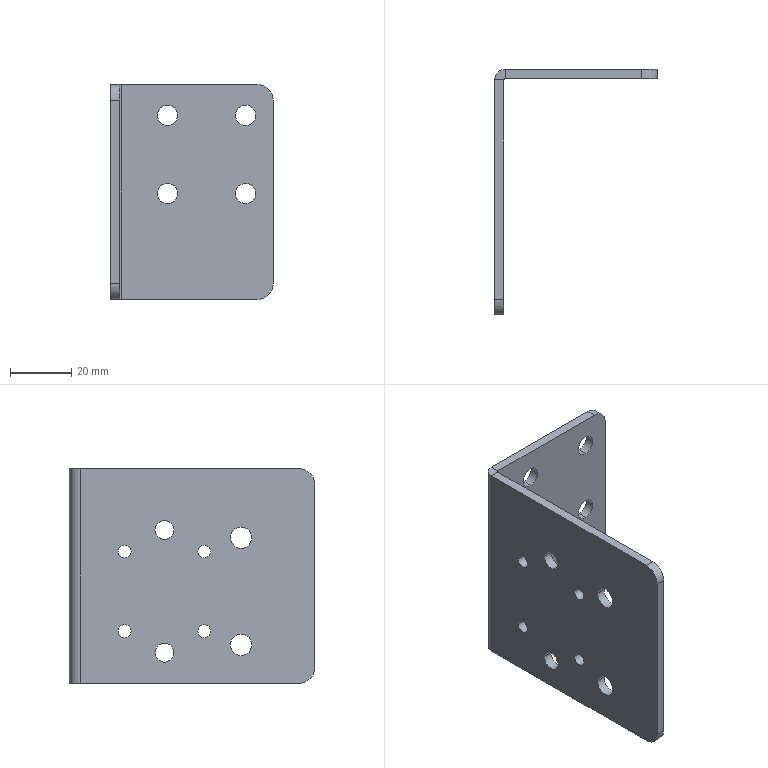Part | SolidWorks | features ICE 11, Fillet 2, ExtruThin 1, FlatPattern 1, FlattenBends 1, ProcessBends 1, SheetMetal 1 | 1 solid | 42 faces | box 53 x 80 x 70 mm | volume 26067 mm3 | cylinder 30 | plane 12 | commonest cylinder face diameters 4.2 x8 6.6 x8 7 x5 6.2 x4 10 x4 1 x1
STEP:
#1=CARTESIAN_POINT('',(0.,122.1,20.));
#2=VERTEX_POINT('',#1);
#3=CARTESIAN_POINT('',(0.,115.9,20.));
#4=VERTEX_POINT('',#3);
#5=CARTESIAN_POINT('',(0.,119.,20.));
#6=DIRECTION('',(-1.,0.,0.));
#7=DIRECTION('',(0.,-1.,0.));
#8=AXIS2_PLACEMENT_3D('',#5,#6,#7);
#9=CIRCLE('',#8,3.1);
#10=EDGE_CURVE('',#2,#4,#9,.T.);
#11=ORIENTED_EDGE('',*,*,#10,.T.);
#12=CARTESIAN_POINT('',(3.,115.9,20.));
#13=VERTEX_POINT('',#12);
#14=CARTESIAN_POINT('',(-7.,115.9,20.));
#15=DIRECTION('',(1.,0.,0.));
#16=VECTOR('',#15,1000.);
#17=LINE('',#14,#16);
#18=EDGE_CURVE('',#4,#13,#17,.T.);
#19=ORIENTED_EDGE('',*,*,#18,.T.);
#20=CARTESIAN_POINT('',(3.,122.1,20.));
#21=VERTEX_POINT('',#20);
#22=CARTESIAN_POINT('',(3.,119.,20.));
#23=DIRECTION('',(1.,0.,0.));
#24=DIRECTION('',(0.,1.,0.));
#25=AXIS2_PLACEMENT_3D('',#22,#23,#24);
#26=CIRCLE('',#25,3.1);
#27=EDGE_CURVE('',#13,#21,#26,.T.);
#28=ORIENTED_EDGE('',*,*,#27,.T.);
#29=CARTESIAN_POINT('',(-7.,122.1,20.));
#30=DIRECTION('',(1.,0.,0.));
#31=VECTOR('',#30,1000.);
#32=LINE('',#29,#31);
#33=EDGE_CURVE('',#2,#21,#32,.T.);
#34=ORIENTED_EDGE('',*,*,#33,.F.);
#35=EDGE_LOOP('',(#11,#19,#28,#34));
#36=FACE_OUTER_BOUND('',#35,.T.);
#37=CARTESIAN_POINT('',(-7.,119.,20.));
#38=DIRECTION('',(1.,0.,0.));
#39=DIRECTION('',(0.,1.,0.));
#40=AXIS2_PLACEMENT_3D('',#37,#38,#39);
#41=CYLINDRICAL_SURFACE('',#40,3.1);
#42=ADVANCED_FACE('',(#36),#41,.F.);
#43=CARTESIAN_POINT('',(0.,97.5,17.5));
#44=VERTEX_POINT('',#43);
#45=CARTESIAN_POINT('',(0.,90.5,17.5));
#46=VERTEX_POINT('',#45);
#47=CARTESIAN_POINT('',(0.,94.,17.5));
#48=DIRECTION('',(-1.,0.,0.));
#49=DIRECTION('',(0.,-1.,0.));
#50=AXIS2_PLACEMENT_3D('',#47,#48,#49);
#51=CIRCLE('',#50,3.5);
#52=EDGE_CURVE('',#44,#46,#51,.T.);
#53=ORIENTED_EDGE('',*,*,#52,.T.);
#54=CARTESIAN_POINT('',(3.,90.5,17.5));
#55=VERTEX_POINT('',#54);
#56=CARTESIAN_POINT('',(-7.,90.5,17.5));
#57=DIRECTION('',(1.,0.,0.));
#58=VECTOR('',#57,1000.);
#59=LINE('',#56,#58);
#60=EDGE_CURVE('',#46,#55,#59,.T.);
#61=ORIENTED_EDGE('',*,*,#60,.T.);
#62=CARTESIAN_POINT('',(3.,97.5,17.5));
#63=VERTEX_POINT('',#62);
#64=CARTESIAN_POINT('',(3.,94.,17.5));
#65=DIRECTION('',(1.,0.,0.));
#66=DIRECTION('',(0.,1.,0.));
#67=AXIS2_PLACEMENT_3D('',#64,#65,#66);
#68=CIRCLE('',#67,3.5);
#69=EDGE_CURVE('',#55,#63,#68,.T.);
#70=ORIENTED_EDGE('',*,*,#69,.T.);
#71=CARTESIAN_POINT('',(-7.,97.5,17.5));
#72=DIRECTION('',(1.,0.,0.));
#73=VECTOR('',#72,1000.);
#74=LINE('',#71,#73);
#75=EDGE_CURVE('',#44,#63,#74,.T.);
#76=ORIENTED_EDGE('',*,*,#75,.F.);
#77=EDGE_LOOP('',(#53,#61,#70,#76));
#78=FACE_OUTER_BOUND('',#77,.T.);
#79=CARTESIAN_POINT('',(-7.,94.,17.5));
#80=DIRECTION('',(1.,0.,0.));
#81=DIRECTION('',(0.,1.,0.));
#82=AXIS2_PLACEMENT_3D('',#79,#80,#81);
#83=CYLINDRICAL_SURFACE('',#82,3.5);
#84=ADVANCED_FACE('',(#78),#83,.F.);
#85=CARTESIAN_POINT('',(0.,97.5,-17.5));
#86=VERTEX_POINT('',#85);
#87=CARTESIAN_POINT('',(0.,90.5,-17.5));
#88=VERTEX_POINT('',#87);
#89=CARTESIAN_POINT('',(0.,94.,-17.5));
#90=DIRECTION('',(-1.,0.,0.));
#91=DIRECTION('',(0.,-1.,0.));
#92=AXIS2_PLACEMENT_3D('',#89,#90,#91);
#93=CIRCLE('',#92,3.5);
#94=EDGE_CURVE('',#86,#88,#93,.T.);
#95=ORIENTED_EDGE('',*,*,#94,.T.);
#96=CARTESIAN_POINT('',(3.,90.5,-17.5));
#97=VERTEX_POINT('',#96);
#98=CARTESIAN_POINT('',(-7.,90.5,-17.5));
#99=DIRECTION('',(1.,0.,0.));
#100=VECTOR('',#99,1000.);
#101=LINE('',#98,#100);
#102=EDGE_CURVE('',#88,#97,#101,.T.);
#103=ORIENTED_EDGE('',*,*,#102,.T.);
#104=CARTESIAN_POINT('',(3.,97.5,-17.5));
#105=VERTEX_POINT('',#104);
#106=CARTESIAN_POINT('',(3.,94.,-17.5));
#107=DIRECTION('',(1.,0.,0.));
#108=DIRECTION('',(0.,1.,0.));
#109=AXIS2_PLACEMENT_3D('',#106,#107,#108);
#110=CIRCLE('',#109,3.5);
#111=EDGE_CURVE('',#97,#105,#110,.T.);
#112=ORIENTED_EDGE('',*,*,#111,.T.);
#113=CARTESIAN_POINT('',(-7.,97.5,-17.5));
#114=DIRECTION('',(1.,0.,0.));
#115=VECTOR('',#114,1000.);
#116=LINE('',#113,#115);
#117=EDGE_CURVE('',#86,#105,#116,.T.);
#118=ORIENTED_EDGE('',*,*,#117,.F.);
#119=EDGE_LOOP('',(#95,#103,#112,#118));
#120=FACE_OUTER_BOUND('',#119,.T.);
#121=CARTESIAN_POINT('',(-7.,94.,-17.5));
#122=DIRECTION('',(1.,0.,0.));
#123=DIRECTION('',(0.,1.,0.));
#124=AXIS2_PLACEMENT_3D('',#121,#122,#123);
#125=CYLINDRICAL_SURFACE('',#124,3.5);
#126=ADVANCED_FACE('',(#120),#125,.F.);
#127=CARTESIAN_POINT('',(0.,122.1,-20.));
#128=VERTEX_POINT('',#127);
#129=CARTESIAN_POINT('',(0.,115.9,-20.));
#130=VERTEX_POINT('',#129);
#131=CARTESIAN_POINT('',(0.,119.,-20.));
#132=DIRECTION('',(-1.,0.,0.));
#133=DIRECTION('',(0.,-1.,0.));
#134=AXIS2_PLACEMENT_3D('',#131,#132,#133);
#135=CIRCLE('',#134,3.1);
#136=EDGE_CURVE('',#128,#130,#135,.T.);
#137=ORIENTED_EDGE('',*,*,#136,.T.);
#138=CARTESIAN_POINT('',(3.,115.9,-20.));
#139=VERTEX_POINT('',#138);
#140=CARTESIAN_POINT('',(-7.,115.9,-20.));
#141=DIRECTION('',(1.,0.,0.));
#142=VECTOR('',#141,1000.);
#143=LINE('',#140,#142);
#144=EDGE_CURVE('',#130,#139,#143,.T.);
#145=ORIENTED_EDGE('',*,*,#144,.T.);
#146=CARTESIAN_POINT('',(3.,122.1,-20.));
#147=VERTEX_POINT('',#146);
#148=CARTESIAN_POINT('',(3.,119.,-20.));
#149=DIRECTION('',(1.,0.,0.));
#150=DIRECTION('',(0.,1.,0.));
#151=AXIS2_PLACEMENT_3D('',#148,#149,#150);
#152=CIRCLE('',#151,3.1);
#153=EDGE_CURVE('',#139,#147,#152,.T.);
#154=ORIENTED_EDGE('',*,*,#153,.T.);
#155=CARTESIAN_POINT('',(-7.,122.1,-20.));
#156=DIRECTION('',(1.,0.,0.));
#157=VECTOR('',#156,1000.);
#158=LINE('',#155,#157);
#159=EDGE_CURVE('',#128,#147,#158,.T.);
#160=ORIENTED_EDGE('',*,*,#159,.F.);
#161=EDGE_LOOP('',(#137,#145,#154,#160));
#162=FACE_OUTER_BOUND('',#161,.T.);
#163=CARTESIAN_POINT('',(-7.,119.,-20.));
#164=DIRECTION('',(1.,0.,0.));
#165=DIRECTION('',(0.,1.,0.));
#166=AXIS2_PLACEMENT_3D('',#163,#164,#165);
#167=CYLINDRICAL_SURFACE('',#166,3.1);
#168=ADVANCED_FACE('',(#162),#167,.F.);
#169=CARTESIAN_POINT('',(0.,108.1,13.));
#170=VERTEX_POINT('',#169);
#171=CARTESIAN_POINT('',(0.,103.9,13.));
#172=VERTEX_POINT('',#171);
#173=CARTESIAN_POINT('',(0.,106.,13.));
#174=DIRECTION('',(-1.,0.,0.));
#175=DIRECTION('',(0.,-1.,0.));
#176=AXIS2_PLACEMENT_3D('',#173,#174,#175);
#177=CIRCLE('',#176,2.1);
#178=EDGE_CURVE('',#170,#172,#177,.T.);
#179=ORIENTED_EDGE('',*,*,#178,.T.);
#180=CARTESIAN_POINT('',(3.,103.9,13.));
#181=VERTEX_POINT('',#180);
#182=CARTESIAN_POINT('',(-7.,103.9,13.));
#183=DIRECTION('',(1.,0.,0.));
#184=VECTOR('',#183,1000.);
#185=LINE('',#182,#184);
#186=EDGE_CURVE('',#172,#181,#185,.T.);
#187=ORIENTED_EDGE('',*,*,#186,.T.);
#188=CARTESIAN_POINT('',(3.,108.1,13.));
#189=VERTEX_POINT('',#188);
#190=CARTESIAN_POINT('',(3.,106.,13.));
#191=DIRECTION('',(1.,0.,0.));
#192=DIRECTION('',(0.,1.,0.));
#193=AXIS2_PLACEMENT_3D('',#190,#191,#192);
#194=CIRCLE('',#193,2.1);
#195=EDGE_CURVE('',#181,#189,#194,.T.);
#196=ORIENTED_EDGE('',*,*,#195,.T.);
#197=CARTESIAN_POINT('',(-7.,108.1,13.));
#198=DIRECTION('',(1.,0.,0.));
#199=VECTOR('',#198,1000.);
#200=LINE('',#197,#199);
#201=EDGE_CURVE('',#170,#189,#200,.T.);
#202=ORIENTED_EDGE('',*,*,#201,.F.);
#203=EDGE_LOOP('',(#179,#187,#196,#202));
#204=FACE_OUTER_BOUND('',#203,.T.);
#205=CARTESIAN_POINT('',(-7.,106.,13.));
#206=DIRECTION('',(1.,0.,0.));
#207=DIRECTION('',(0.,1.,0.));
#208=AXIS2_PLACEMENT_3D('',#205,#206,#207);
#209=CYLINDRICAL_SURFACE('',#208,2.1);
#210=ADVANCED_FACE('',(#204),#209,.F.);
#211=CARTESIAN_POINT('',(0.,108.1,-13.));
#212=VERTEX_POINT('',#211);
#213=CARTESIAN_POINT('',(0.,103.9,-13.));
#214=VERTEX_POINT('',#213);
#215=CARTESIAN_POINT('',(0.,106.,-13.));
#216=DIRECTION('',(-1.,0.,0.));
#217=DIRECTION('',(0.,-1.,0.));
#218=AXIS2_PLACEMENT_3D('',#215,#216,#217);
#219=CIRCLE('',#218,2.1);
#220=EDGE_CURVE('',#212,#214,#219,.T.);
#221=ORIENTED_EDGE('',*,*,#220,.T.);
#222=CARTESIAN_POINT('',(3.,103.9,-13.));
#223=VERTEX_POINT('',#222);
#224=CARTESIAN_POINT('',(-7.,103.9,-13.));
#225=DIRECTION('',(1.,0.,0.));
#226=VECTOR('',#225,1000.);
#227=LINE('',#224,#226);
#228=EDGE_CURVE('',#214,#223,#227,.T.);
#229=ORIENTED_EDGE('',*,*,#228,.T.);
#230=CARTESIAN_POINT('',(3.,108.1,-13.));
#231=VERTEX_POINT('',#230);
#232=CARTESIAN_POINT('',(3.,106.,-13.));
#233=DIRECTION('',(1.,0.,0.));
#234=DIRECTION('',(0.,1.,0.));
#235=AXIS2_PLACEMENT_3D('',#232,#233,#234);
#236=CIRCLE('',#235,2.1);
#237=EDGE_CURVE('',#223,#231,#236,.T.);
#238=ORIENTED_EDGE('',*,*,#237,.T.);
#239=CARTESIAN_POINT('',(-7.,108.1,-13.));
#240=DIRECTION('',(1.,0.,0.));
#241=VECTOR('',#240,1000.);
#242=LINE('',#239,#241);
#243=EDGE_CURVE('',#212,#231,#242,.T.);
#244=ORIENTED_EDGE('',*,*,#243,.F.);
#245=EDGE_LOOP('',(#221,#229,#238,#244));
#246=FACE_OUTER_BOUND('',#245,.T.);
#247=CARTESIAN_POINT('',(-7.,106.,-13.));
#248=DIRECTION('',(1.,0.,0.));
#249=DIRECTION('',(0.,1.,0.));
#250=AXIS2_PLACEMENT_3D('',#247,#248,#249);
#251=CYLINDRICAL_SURFACE('',#250,2.1);
#252=ADVANCED_FACE('',(#246),#251,.F.);
#253=CARTESIAN_POINT('',(0.,134.1,-13.));
#254=VERTEX_POINT('',#253);
#255=CARTESIAN_POINT('',(0.,129.9,-13.));
#256=VERTEX_POINT('',#255);
#257=CARTESIAN_POINT('',(0.,132.,-13.));
#258=DIRECTION('',(-1.,0.,0.));
#259=DIRECTION('',(0.,-1.,0.));
#260=AXIS2_PLACEMENT_3D('',#257,#258,#259);
#261=CIRCLE('',#260,2.1);
#262=EDGE_CURVE('',#254,#256,#261,.T.);
#263=ORIENTED_EDGE('',*,*,#262,.T.);
#264=CARTESIAN_POINT('',(3.,129.9,-13.));
#265=VERTEX_POINT('',#264);
#266=CARTESIAN_POINT('',(-7.,129.9,-13.));
#267=DIRECTION('',(1.,0.,0.));
#268=VECTOR('',#267,1000.);
#269=LINE('',#266,#268);
#270=EDGE_CURVE('',#256,#265,#269,.T.);
#271=ORIENTED_EDGE('',*,*,#270,.T.);
#272=CARTESIAN_POINT('',(3.,134.1,-13.));
#273=VERTEX_POINT('',#272);
#274=CARTESIAN_POINT('',(3.,132.,-13.));
#275=DIRECTION('',(1.,0.,0.));
#276=DIRECTION('',(0.,1.,0.));
#277=AXIS2_PLACEMENT_3D('',#274,#275,#276);
#278=CIRCLE('',#277,2.1);
#279=EDGE_CURVE('',#265,#273,#278,.T.);
#280=ORIENTED_EDGE('',*,*,#279,.T.);
#281=CARTESIAN_POINT('',(-7.,134.1,-13.));
#282=DIRECTION('',(1.,0.,0.));
#283=VECTOR('',#282,1000.);
#284=LINE('',#281,#283);
#285=EDGE_CURVE('',#254,#273,#284,.T.);
#286=ORIENTED_EDGE('',*,*,#285,.F.);
#287=EDGE_LOOP('',(#263,#271,#280,#286));
#288=FACE_OUTER_BOUND('',#287,.T.);
#289=CARTESIAN_POINT('',(-7.,132.,-13.));
#290=DIRECTION('',(1.,0.,0.));
#291=DIRECTION('',(0.,1.,0.));
#292=AXIS2_PLACEMENT_3D('',#289,#290,#291);
#293=CYLINDRICAL_SURFACE('',#292,2.1);
#294=ADVANCED_FACE('',(#288),#293,.F.);
#295=CARTESIAN_POINT('',(0.,134.1,13.));
#296=VERTEX_POINT('',#295);
#297=CARTESIAN_POINT('',(0.,129.9,13.));
#298=VERTEX_POINT('',#297);
#299=CARTESIAN_POINT('',(0.,132.,13.));
#300=DIRECTION('',(-1.,0.,0.));
#301=DIRECTION('',(0.,-1.,0.));
#302=AXIS2_PLACEMENT_3D('',#299,#300,#301);
#303=CIRCLE('',#302,2.1);
#304=EDGE_CURVE('',#296,#298,#303,.T.);
#305=ORIENTED_EDGE('',*,*,#304,.T.);
#306=CARTESIAN_POINT('',(3.,129.9,13.));
#307=VERTEX_POINT('',#306);
#308=CARTESIAN_POINT('',(-7.,129.9,13.));
#309=DIRECTION('',(1.,0.,0.));
#310=VECTOR('',#309,1000.);
#311=LINE('',#308,#310);
#312=EDGE_CURVE('',#298,#307,#311,.T.);
#313=ORIENTED_EDGE('',*,*,#312,.T.);
#314=CARTESIAN_POINT('',(3.,134.1,13.));
#315=VERTEX_POINT('',#314);
#316=CARTESIAN_POINT('',(3.,132.,13.));
#317=DIRECTION('',(1.,0.,0.));
#318=DIRECTION('',(0.,1.,0.));
#319=AXIS2_PLACEMENT_3D('',#316,#317,#318);
#320=CIRCLE('',#319,2.1);
#321=EDGE_CURVE('',#307,#315,#320,.T.);
#322=ORIENTED_EDGE('',*,*,#321,.T.);
#323=CARTESIAN_POINT('',(-7.,134.1,13.));
#324=DIRECTION('',(1.,0.,0.));
#325=VECTOR('',#324,1000.);
#326=LINE('',#323,#325);
#327=EDGE_CURVE('',#296,#315,#326,.T.);
#328=ORIENTED_EDGE('',*,*,#327,.F.);
#329=EDGE_LOOP('',(#305,#313,#322,#328));
#330=FACE_OUTER_BOUND('',#329,.T.);
#331=CARTESIAN_POINT('',(-7.,132.,13.));
#332=DIRECTION('',(1.,0.,0.));
#333=DIRECTION('',(0.,1.,0.));
#334=AXIS2_PLACEMENT_3D('',#331,#332,#333);
#335=CYLINDRICAL_SURFACE('',#334,2.1);
#336=ADVANCED_FACE('',(#330),#335,.F.);
#337=CARTESIAN_POINT('',(44.,147.,26.7));
#338=VERTEX_POINT('',#337);
#339=CARTESIAN_POINT('',(44.,147.,33.3));
#340=VERTEX_POINT('',#339);
#341=CARTESIAN_POINT('',(44.,147.,30.));
#342=DIRECTION('',(0.,1.,0.));
#343=DIRECTION('',(-1.,0.,0.));
#344=AXIS2_PLACEMENT_3D('',#341,#342,#343);
#345=CIRCLE('',#344,3.3);
#346=EDGE_CURVE('',#338,#340,#345,.T.);
#347=ORIENTED_EDGE('',*,*,#346,.F.);
#348=CARTESIAN_POINT('',(44.,150.,26.7));
#349=VERTEX_POINT('',#348);
#350=CARTESIAN_POINT('',(44.,140.,26.7));
#351=DIRECTION('',(0.,1.,0.));
#352=VECTOR('',#351,1000.);
#353=LINE('',#350,#352);
#354=EDGE_CURVE('',#338,#349,#353,.T.);
#355=ORIENTED_EDGE('',*,*,#354,.T.);
#356=CARTESIAN_POINT('',(44.,150.,33.3));
#357=VERTEX_POINT('',#356);
#358=CARTESIAN_POINT('',(44.,150.,30.));
#359=DIRECTION('',(0.,1.,0.));
#360=DIRECTION('',(0.,0.,1.));
#361=AXIS2_PLACEMENT_3D('',#358,#359,#360);
#362=CIRCLE('',#361,3.3);
#363=EDGE_CURVE('',#349,#357,#362,.T.);
#364=ORIENTED_EDGE('',*,*,#363,.T.);
#365=CARTESIAN_POINT('',(44.,140.,33.3));
#366=DIRECTION('',(0.,1.,0.));
#367=VECTOR('',#366,1000.);
#368=LINE('',#365,#367);
#369=EDGE_CURVE('',#340,#357,#368,.T.);
#370=ORIENTED_EDGE('',*,*,#369,.F.);
#371=EDGE_LOOP('',(#347,#355,#364,#370));
#372=FACE_OUTER_BOUND('',#371,.T.);
#373=CARTESIAN_POINT('',(44.,140.,30.));
#374=DIRECTION('',(0.,1.,0.));
#375=DIRECTION('',(0.,0.,1.));
#376=AXIS2_PLACEMENT_3D('',#373,#374,#375);
#377=CYLINDRICAL_SURFACE('',#376,3.3);
#378=ADVANCED_FACE('',(#372),#377,.F.);
#379=CARTESIAN_POINT('',(44.,147.,1.2));
#380=VERTEX_POINT('',#379);
#381=CARTESIAN_POINT('',(44.,147.,7.8));
#382=VERTEX_POINT('',#381);
#383=CARTESIAN_POINT('',(44.,147.,4.5));
#384=DIRECTION('',(0.,1.,0.));
#385=DIRECTION('',(-1.,0.,0.));
#386=AXIS2_PLACEMENT_3D('',#383,#384,#385);
#387=CIRCLE('',#386,3.3);
#388=EDGE_CURVE('',#380,#382,#387,.T.);
#389=ORIENTED_EDGE('',*,*,#388,.F.);
#390=CARTESIAN_POINT('',(44.,150.,1.2));
#391=VERTEX_POINT('',#390);
#392=CARTESIAN_POINT('',(44.,140.,1.2));
#393=DIRECTION('',(0.,1.,0.));
#394=VECTOR('',#393,1000.);
#395=LINE('',#392,#394);
#396=EDGE_CURVE('',#380,#391,#395,.T.);
#397=ORIENTED_EDGE('',*,*,#396,.T.);
#398=CARTESIAN_POINT('',(44.,150.,7.8));
#399=VERTEX_POINT('',#398);
#400=CARTESIAN_POINT('',(44.,150.,4.5));
#401=DIRECTION('',(0.,1.,0.));
#402=DIRECTION('',(0.,0.,1.));
#403=AXIS2_PLACEMENT_3D('',#400,#401,#402);
#404=CIRCLE('',#403,3.3);
#405=EDGE_CURVE('',#391,#399,#404,.T.);
#406=ORIENTED_EDGE('',*,*,#405,.T.);
#407=CARTESIAN_POINT('',(44.,140.,7.8));
#408=DIRECTION('',(0.,1.,0.));
#409=VECTOR('',#408,1000.);
#410=LINE('',#407,#409);
#411=EDGE_CURVE('',#382,#399,#410,.T.);
#412=ORIENTED_EDGE('',*,*,#411,.F.);
#413=EDGE_LOOP('',(#389,#397,#406,#412));
#414=FACE_OUTER_BOUND('',#413,.T.);
#415=CARTESIAN_POINT('',(44.,140.,4.5));
#416=DIRECTION('',(0.,1.,0.));
#417=DIRECTION('',(0.,0.,1.));
#418=AXIS2_PLACEMENT_3D('',#415,#416,#417);
#419=CYLINDRICAL_SURFACE('',#418,3.3);
#420=ADVANCED_FACE('',(#414),#419,.F.);
#421=CARTESIAN_POINT('',(18.5,147.,1.2));
#422=VERTEX_POINT('',#421);
#423=CARTESIAN_POINT('',(18.5,147.,7.8));
#424=VERTEX_POINT('',#423);
#425=CARTESIAN_POINT('',(18.5,147.,4.5));
#426=DIRECTION('',(0.,1.,0.));
#427=DIRECTION('',(-1.,0.,0.));
#428=AXIS2_PLACEMENT_3D('',#425,#426,#427);
#429=CIRCLE('',#428,3.3);
#430=EDGE_CURVE('',#422,#424,#429,.T.);
#431=ORIENTED_EDGE('',*,*,#430,.F.);
#432=CARTESIAN_POINT('',(18.5,150.,1.2));
#433=VERTEX_POINT('',#432);
#434=CARTESIAN_POINT('',(18.5,140.,1.2));
#435=DIRECTION('',(0.,1.,0.));
#436=VECTOR('',#435,1000.);
#437=LINE('',#434,#436);
#438=EDGE_CURVE('',#422,#433,#437,.T.);
#439=ORIENTED_EDGE('',*,*,#438,.T.);
#440=CARTESIAN_POINT('',(18.5,150.,7.8));
#441=VERTEX_POINT('',#440);
#442=CARTESIAN_POINT('',(18.5,150.,4.5));
#443=DIRECTION('',(0.,1.,0.));
#444=DIRECTION('',(0.,0.,1.));
#445=AXIS2_PLACEMENT_3D('',#442,#443,#444);
#446=CIRCLE('',#445,3.3);
#447=EDGE_CURVE('',#433,#441,#446,.T.);
#448=ORIENTED_EDGE('',*,*,#447,.T.);
#449=CARTESIAN_POINT('',(18.5,140.,7.8));
#450=DIRECTION('',(0.,1.,0.));
#451=VECTOR('',#450,1000.);
#452=LINE('',#449,#451);
#453=EDGE_CURVE('',#424,#441,#452,.T.);
#454=ORIENTED_EDGE('',*,*,#453,.F.);
#455=EDGE_LOOP('',(#431,#439,#448,#454));
#456=FACE_OUTER_BOUND('',#455,.T.);
#457=CARTESIAN_POINT('',(18.5,140.,4.5));
#458=DIRECTION('',(0.,1.,0.));
#459=DIRECTION('',(0.,0.,1.));
#460=AXIS2_PLACEMENT_3D('',#457,#458,#459);
#461=CYLINDRICAL_SURFACE('',#460,3.3);
#462=ADVANCED_FACE('',(#456),#461,.F.);
#463=CARTESIAN_POINT('',(18.5,147.,26.7));
#464=VERTEX_POINT('',#463);
#465=CARTESIAN_POINT('',(18.5,147.,33.3));
#466=VERTEX_POINT('',#465);
#467=CARTESIAN_POINT('',(18.5,147.,30.));
#468=DIRECTION('',(0.,1.,0.));
#469=DIRECTION('',(-1.,0.,0.));
#470=AXIS2_PLACEMENT_3D('',#467,#468,#469);
#471=CIRCLE('',#470,3.3);
#472=EDGE_CURVE('',#464,#466,#471,.T.);
#473=ORIENTED_EDGE('',*,*,#472,.F.);
#474=CARTESIAN_POINT('',(18.5,150.,26.7));
#475=VERTEX_POINT('',#474);
#476=CARTESIAN_POINT('',(18.5,140.,26.7));
#477=DIRECTION('',(0.,1.,0.));
#478=VECTOR('',#477,1000.);
#479=LINE('',#476,#478);
#480=EDGE_CURVE('',#464,#475,#479,.T.);
#481=ORIENTED_EDGE('',*,*,#480,.T.);
#482=CARTESIAN_POINT('',(18.5,150.,33.3));
#483=VERTEX_POINT('',#482);
#484=CARTESIAN_POINT('',(18.5,150.,30.));
#485=DIRECTION('',(0.,1.,0.));
#486=DIRECTION('',(0.,0.,1.));
#487=AXIS2_PLACEMENT_3D('',#484,#485,#486);
#488=CIRCLE('',#487,3.3);
#489=EDGE_CURVE('',#475,#483,#488,.T.);
#490=ORIENTED_EDGE('',*,*,#489,.T.);
#491=CARTESIAN_POINT('',(18.5,140.,33.3));
#492=DIRECTION('',(0.,1.,0.));
#493=VECTOR('',#492,1000.);
#494=LINE('',#491,#493);
#495=EDGE_CURVE('',#466,#483,#494,.T.);
#496=ORIENTED_EDGE('',*,*,#495,.F.);
#497=EDGE_LOOP('',(#473,#481,#490,#496));
#498=FACE_OUTER_BOUND('',#497,.T.);
#499=CARTESIAN_POINT('',(18.5,140.,30.));
#500=DIRECTION('',(0.,1.,0.));
#501=DIRECTION('',(0.,0.,1.));
#502=AXIS2_PLACEMENT_3D('',#499,#500,#501);
#503=CYLINDRICAL_SURFACE('',#502,3.3);
#504=ADVANCED_FACE('',(#498),#503,.F.);
#505=ORIENTED_EDGE('',*,*,#480,.F.);
#506=CARTESIAN_POINT('',(18.5,147.,30.));
#507=DIRECTION('',(0.,1.,0.));
#508=DIRECTION('',(-1.,0.,0.));
#509=AXIS2_PLACEMENT_3D('',#506,#507,#508);
#510=CIRCLE('',#509,3.3);
#511=EDGE_CURVE('',#466,#464,#510,.T.);
#512=ORIENTED_EDGE('',*,*,#511,.F.);
#513=ORIENTED_EDGE('',*,*,#495,.T.);
#514=CARTESIAN_POINT('',(18.5,150.,30.));
#515=DIRECTION('',(0.,1.,0.));
#516=DIRECTION('',(0.,0.,1.));
#517=AXIS2_PLACEMENT_3D('',#514,#515,#516);
#518=CIRCLE('',#517,3.3);
#519=EDGE_CURVE('',#483,#475,#518,.T.);
#520=ORIENTED_EDGE('',*,*,#519,.T.);
#521=EDGE_LOOP('',(#505,#512,#513,#520));
#522=FACE_OUTER_BOUND('',#521,.T.);
#523=CARTESIAN_POINT('',(18.5,140.,30.));
#524=DIRECTION('',(0.,1.,0.));
#525=DIRECTION('',(0.,0.,1.));
#526=AXIS2_PLACEMENT_3D('',#523,#524,#525);
#527=CYLINDRICAL_SURFACE('',#526,3.3);
#528=ADVANCED_FACE('',(#522),#527,.F.);
#529=ORIENTED_EDGE('',*,*,#438,.F.);
#530=CARTESIAN_POINT('',(18.5,147.,4.5));
#531=DIRECTION('',(0.,1.,0.));
#532=DIRECTION('',(-1.,0.,0.));
#533=AXIS2_PLACEMENT_3D('',#530,#531,#532);
#534=CIRCLE('',#533,3.3);
#535=EDGE_CURVE('',#424,#422,#534,.T.);
#536=ORIENTED_EDGE('',*,*,#535,.F.);
#537=ORIENTED_EDGE('',*,*,#453,.T.);
#538=CARTESIAN_POINT('',(18.5,150.,4.5));
#539=DIRECTION('',(0.,1.,0.));
#540=DIRECTION('',(0.,0.,1.));
#541=AXIS2_PLACEMENT_3D('',#538,#539,#540);
#542=CIRCLE('',#541,3.3);
#543=EDGE_CURVE('',#441,#433,#542,.T.);
#544=ORIENTED_EDGE('',*,*,#543,.T.);
#545=EDGE_LOOP('',(#529,#536,#537,#544));
#546=FACE_OUTER_BOUND('',#545,.T.);
#547=CARTESIAN_POINT('',(18.5,140.,4.5));
#548=DIRECTION('',(0.,1.,0.));
#549=DIRECTION('',(0.,0.,1.));
#550=AXIS2_PLACEMENT_3D('',#547,#548,#549);
#551=CYLINDRICAL_SURFACE('',#550,3.3);
#552=ADVANCED_FACE('',(#546),#551,.F.);
#553=ORIENTED_EDGE('',*,*,#396,.F.);
#554=CARTESIAN_POINT('',(44.,147.,4.5));
#555=DIRECTION('',(0.,1.,0.));
#556=DIRECTION('',(-1.,0.,0.));
#557=AXIS2_PLACEMENT_3D('',#554,#555,#556);
#558=CIRCLE('',#557,3.3);
#559=EDGE_CURVE('',#382,#380,#558,.T.);
#560=ORIENTED_EDGE('',*,*,#559,.F.);
#561=ORIENTED_EDGE('',*,*,#411,.T.);
#562=CARTESIAN_POINT('',(44.,150.,4.5));
#563=DIRECTION('',(0.,1.,0.));
#564=DIRECTION('',(0.,0.,1.));
#565=AXIS2_PLACEMENT_3D('',#562,#563,#564);
#566=CIRCLE('',#565,3.3);
#567=EDGE_CURVE('',#399,#391,#566,.T.);
#568=ORIENTED_EDGE('',*,*,#567,.T.);
#569=EDGE_LOOP('',(#553,#560,#561,#568));
#570=FACE_OUTER_BOUND('',#569,.T.);
#571=CARTESIAN_POINT('',(44.,140.,4.5));
#572=DIRECTION('',(0.,1.,0.));
#573=DIRECTION('',(0.,0.,1.));
#574=AXIS2_PLACEMENT_3D('',#571,#572,#573);
#575=CYLINDRICAL_SURFACE('',#574,3.3);
#576=ADVANCED_FACE('',(#570),#575,.F.);
#577=ORIENTED_EDGE('',*,*,#354,.F.);
#578=CARTESIAN_POINT('',(44.,147.,30.));
#579=DIRECTION('',(0.,1.,0.));
#580=DIRECTION('',(-1.,0.,0.));
#581=AXIS2_PLACEMENT_3D('',#578,#579,#580);
#582=CIRCLE('',#581,3.3);
#583=EDGE_CURVE('',#340,#338,#582,.T.);
#584=ORIENTED_EDGE('',*,*,#583,.F.);
#585=ORIENTED_EDGE('',*,*,#369,.T.);
#586=CARTESIAN_POINT('',(44.,150.,30.));
#587=DIRECTION('',(0.,1.,0.));
#588=DIRECTION('',(0.,0.,1.));
#589=AXIS2_PLACEMENT_3D('',#586,#587,#588);
#590=CIRCLE('',#589,3.3);
#591=EDGE_CURVE('',#357,#349,#590,.T.);
#592=ORIENTED_EDGE('',*,*,#591,.T.);
#593=EDGE_LOOP('',(#577,#584,#585,#592));
#594=FACE_OUTER_BOUND('',#593,.T.);
#595=CARTESIAN_POINT('',(44.,140.,30.));
#596=DIRECTION('',(0.,1.,0.));
#597=DIRECTION('',(0.,0.,1.));
#598=AXIS2_PLACEMENT_3D('',#595,#596,#597);
#599=CYLINDRICAL_SURFACE('',#598,3.3);
#600=ADVANCED_FACE('',(#594),#599,.F.);
#601=CARTESIAN_POINT('',(53.,147.,-25.));
#602=VERTEX_POINT('',#601);
#603=CARTESIAN_POINT('',(53.,150.,-25.));
#604=VERTEX_POINT('',#603);
#605=CARTESIAN_POINT('',(53.,-21.467,-25.));
#606=DIRECTION('',(0.,1.,0.));
#607=VECTOR('',#606,1000.);
#608=LINE('',#605,#607);
#609=EDGE_CURVE('',#602,#604,#608,.T.);
#610=ORIENTED_EDGE('',*,*,#609,.T.);
#611=CARTESIAN_POINT('',(53.,150.,35.));
#612=VERTEX_POINT('',#611);
#613=CARTESIAN_POINT('',(53.,150.,30.));
#614=DIRECTION('',(0.,0.,1.));
#615=VECTOR('',#614,1000.);
#616=LINE('',#613,#615);
#617=EDGE_CURVE('',#604,#612,#616,.T.);
#618=ORIENTED_EDGE('',*,*,#617,.T.);
#619=CARTESIAN_POINT('',(53.,147.,35.));
#620=VERTEX_POINT('',#619);
#621=CARTESIAN_POINT('',(53.,-21.467,35.));
#622=DIRECTION('',(0.,1.,0.));
#623=VECTOR('',#622,1000.);
#624=LINE('',#621,#623);
#625=EDGE_CURVE('',#620,#612,#624,.T.);
#626=ORIENTED_EDGE('',*,*,#625,.F.);
#627=CARTESIAN_POINT('',(53.,147.,30.));
#628=DIRECTION('',(0.,0.,-1.));
#629=VECTOR('',#628,1000.);
#630=LINE('',#627,#629);
#631=EDGE_CURVE('',#620,#602,#630,.T.);
#632=ORIENTED_EDGE('',*,*,#631,.T.);
#633=EDGE_LOOP('',(#610,#618,#626,#632));
#634=FACE_OUTER_BOUND('',#633,.T.);
#635=CARTESIAN_POINT('',(53.,-21.467,30.));
#636=DIRECTION('',(1.,0.,0.));
#637=DIRECTION('',(0.,1.,0.));
#638=AXIS2_PLACEMENT_3D('',#635,#636,#637);
#639=PLANE('',#638);
#640=ADVANCED_FACE('',(#634),#639,.T.);
#641=CARTESIAN_POINT('',(48.,150.,40.));
#642=VERTEX_POINT('',#641);
#643=CARTESIAN_POINT('',(48.,150.,35.));
#644=DIRECTION('',(0.,1.,0.));
#645=DIRECTION('',(0.,0.,1.));
#646=AXIS2_PLACEMENT_3D('',#643,#644,#645);
#647=CIRCLE('',#646,5.);
#648=EDGE_CURVE('',#642,#612,#647,.T.);
#649=ORIENTED_EDGE('',*,*,#648,.F.);
#650=CARTESIAN_POINT('',(48.,147.,40.));
#651=VERTEX_POINT('',#650);
#652=CARTESIAN_POINT('',(48.,-21.467,40.));
#653=DIRECTION('',(0.,1.,0.));
#654=VECTOR('',#653,1000.);
#655=LINE('',#652,#654);
#656=EDGE_CURVE('',#651,#642,#655,.T.);
#657=ORIENTED_EDGE('',*,*,#656,.F.);
#658=CARTESIAN_POINT('',(48.,147.,35.));
#659=DIRECTION('',(0.,-1.,0.));
#660=DIRECTION('',(-1.,0.,0.));
#661=AXIS2_PLACEMENT_3D('',#658,#659,#660);
#662=CIRCLE('',#661,5.);
#663=EDGE_CURVE('',#620,#651,#662,.T.);
#664=ORIENTED_EDGE('',*,*,#663,.F.);
#665=ORIENTED_EDGE('',*,*,#625,.T.);
#666=EDGE_LOOP('',(#649,#657,#664,#665));
#667=FACE_OUTER_BOUND('',#666,.T.);
#668=CARTESIAN_POINT('',(48.,-21.467,35.));
#669=DIRECTION('',(0.,1.,0.));
#670=DIRECTION('',(-1.,0.,0.));
#671=AXIS2_PLACEMENT_3D('',#668,#669,#670);
#672=CYLINDRICAL_SURFACE('',#671,5.);
#673=ADVANCED_FACE('',(#667),#672,.T.);
#674=CARTESIAN_POINT('',(48.,150.,-30.));
#675=VERTEX_POINT('',#674);
#676=CARTESIAN_POINT('',(48.,150.,-25.));
#677=DIRECTION('',(0.,1.,0.));
#678=DIRECTION('',(0.,0.,1.));
#679=AXIS2_PLACEMENT_3D('',#676,#677,#678);
#680=CIRCLE('',#679,5.);
#681=EDGE_CURVE('',#604,#675,#680,.T.);
#682=ORIENTED_EDGE('',*,*,#681,.F.);
#683=ORIENTED_EDGE('',*,*,#609,.F.);
#684=CARTESIAN_POINT('',(48.,147.,-30.));
#685=VERTEX_POINT('',#684);
#686=CARTESIAN_POINT('',(48.,147.,-25.));
#687=DIRECTION('',(0.,-1.,0.));
#688=DIRECTION('',(-1.,0.,0.));
#689=AXIS2_PLACEMENT_3D('',#686,#687,#688);
#690=CIRCLE('',#689,5.);
#691=EDGE_CURVE('',#685,#602,#690,.T.);
#692=ORIENTED_EDGE('',*,*,#691,.F.);
#693=CARTESIAN_POINT('',(48.,-21.467,-30.));
#694=DIRECTION('',(0.,1.,0.));
#695=VECTOR('',#694,1000.);
#696=LINE('',#693,#695);
#697=EDGE_CURVE('',#685,#675,#696,.T.);
#698=ORIENTED_EDGE('',*,*,#697,.T.);
#699=EDGE_LOOP('',(#682,#683,#692,#698));
#700=FACE_OUTER_BOUND('',#699,.T.);
#701=CARTESIAN_POINT('',(48.,-21.467,-25.));
#702=DIRECTION('',(0.,1.,0.));
#703=DIRECTION('',(-1.,0.,0.));
#704=AXIS2_PLACEMENT_3D('',#701,#702,#703);
#705=CYLINDRICAL_SURFACE('',#704,5.);
#706=ADVANCED_FACE('',(#700),#705,.T.);
#707=CARTESIAN_POINT('',(3.5,147.,-30.));
#708=VERTEX_POINT('',#707);
#709=CARTESIAN_POINT('',(3.5,150.,-30.));
#710=VERTEX_POINT('',#709);
#711=CARTESIAN_POINT('',(3.5,-21.467,-30.));
#712=DIRECTION('',(0.,1.,0.));
#713=VECTOR('',#712,1000.);
#714=LINE('',#711,#713);
#715=EDGE_CURVE('',#708,#710,#714,.T.);
#716=ORIENTED_EDGE('',*,*,#715,.T.);
#717=CARTESIAN_POINT('',(3.,150.,-30.));
#718=DIRECTION('',(-1.,0.,0.));
#719=VECTOR('',#718,1000.);
#720=LINE('',#717,#719);
#721=EDGE_CURVE('',#675,#710,#720,.T.);
#722=ORIENTED_EDGE('',*,*,#721,.F.);
#723=ORIENTED_EDGE('',*,*,#697,.F.);
#724=CARTESIAN_POINT('',(53.,147.,-30.));
#725=DIRECTION('',(-1.,0.,0.));
#726=VECTOR('',#725,1000.);
#727=LINE('',#724,#726);
#728=EDGE_CURVE('',#685,#708,#727,.T.);
#729=ORIENTED_EDGE('',*,*,#728,.T.);
#730=EDGE_LOOP('',(#716,#722,#723,#729));
#731=FACE_OUTER_BOUND('',#730,.T.);
#732=CARTESIAN_POINT('',(53.,-21.467,-30.));
#733=DIRECTION('',(0.,0.,-1.));
#734=DIRECTION('',(0.,1.,0.));
#735=AXIS2_PLACEMENT_3D('',#732,#733,#734);
#736=PLANE('',#735);
#737=ADVANCED_FACE('',(#731),#736,.T.);
#738=CARTESIAN_POINT('',(3.5,150.,40.));
#739=VERTEX_POINT('',#738);
#740=CARTESIAN_POINT('',(3.5,150.,-30.));
#741=DIRECTION('',(0.,0.,-1.));
#742=VECTOR('',#741,1000.);
#743=LINE('',#740,#742);
#744=EDGE_CURVE('',#739,#710,#743,.T.);
#745=ORIENTED_EDGE('',*,*,#744,.F.);
#746=CARTESIAN_POINT('',(53.,150.,40.));
#747=DIRECTION('',(-1.,0.,0.));
#748=VECTOR('',#747,1000.);
#749=LINE('',#746,#748);
#750=EDGE_CURVE('',#642,#739,#749,.T.);
#751=ORIENTED_EDGE('',*,*,#750,.F.);
#752=ORIENTED_EDGE('',*,*,#648,.T.);
#753=ORIENTED_EDGE('',*,*,#617,.F.);
#754=ORIENTED_EDGE('',*,*,#681,.T.);
#755=ORIENTED_EDGE('',*,*,#721,.T.);
#756=EDGE_LOOP('',(#745,#751,#752,#753,#754,#755));
#757=FACE_OUTER_BOUND('',#756,.T.);
#758=ORIENTED_EDGE('',*,*,#591,.F.);
#759=ORIENTED_EDGE('',*,*,#363,.F.);
#760=EDGE_LOOP('',(#758,#759));
#761=FACE_BOUND('',#760,.T.);
#762=ORIENTED_EDGE('',*,*,#567,.F.);
#763=ORIENTED_EDGE('',*,*,#405,.F.);
#764=EDGE_LOOP('',(#762,#763));
#765=FACE_BOUND('',#764,.T.);
#766=ORIENTED_EDGE('',*,*,#543,.F.);
#767=ORIENTED_EDGE('',*,*,#447,.F.);
#768=EDGE_LOOP('',(#766,#767));
#769=FACE_BOUND('',#768,.T.);
#770=ORIENTED_EDGE('',*,*,#519,.F.);
#771=ORIENTED_EDGE('',*,*,#489,.F.);
#772=EDGE_LOOP('',(#770,#771));
#773=FACE_BOUND('',#772,.T.);
#774=CARTESIAN_POINT('',(0.,150.,0.));
#775=DIRECTION('',(0.,1.,0.));
#776=DIRECTION('',(0.,0.,1.));
#777=AXIS2_PLACEMENT_3D('',#774,#775,#776);
#778=PLANE('',#777);
#779=ADVANCED_FACE('',(#757,#761,#765,#769,#773),#778,.T.);
#780=ORIENTED_EDGE('',*,*,#656,.T.);
#781=ORIENTED_EDGE('',*,*,#750,.T.);
#782=CARTESIAN_POINT('',(3.5,147.,40.));
#783=VERTEX_POINT('',#782);
#784=CARTESIAN_POINT('',(3.5,-21.467,40.));
#785=DIRECTION('',(0.,1.,0.));
#786=VECTOR('',#785,1000.);
#787=LINE('',#784,#786);
#788=EDGE_CURVE('',#783,#739,#787,.T.);
#789=ORIENTED_EDGE('',*,*,#788,.F.);
#790=CARTESIAN_POINT('',(3.,147.,40.));
#791=DIRECTION('',(-1.,0.,0.));
#792=VECTOR('',#791,1000.);
#793=LINE('',#790,#792);
#794=EDGE_CURVE('',#651,#783,#793,.T.);
#795=ORIENTED_EDGE('',*,*,#794,.F.);
#796=EDGE_LOOP('',(#780,#781,#789,#795));
#797=FACE_OUTER_BOUND('',#796,.T.);
#798=CARTESIAN_POINT('',(3.,-21.467,40.));
#799=DIRECTION('',(0.,0.,1.));
#800=DIRECTION('',(0.,-1.,0.));
#801=AXIS2_PLACEMENT_3D('',#798,#799,#800);
#802=PLANE('',#801);
#803=ADVANCED_FACE('',(#797),#802,.T.);
#804=ORIENTED_EDGE('',*,*,#583,.T.);
#805=ORIENTED_EDGE('',*,*,#346,.T.);
#806=EDGE_LOOP('',(#804,#805));
#807=FACE_BOUND('',#806,.T.);
#808=ORIENTED_EDGE('',*,*,#559,.T.);
#809=ORIENTED_EDGE('',*,*,#388,.T.);
#810=EDGE_LOOP('',(#808,#809));
#811=FACE_BOUND('',#810,.T.);
#812=ORIENTED_EDGE('',*,*,#535,.T.);
#813=ORIENTED_EDGE('',*,*,#430,.T.);
#814=EDGE_LOOP('',(#812,#813));
#815=FACE_BOUND('',#814,.T.);
#816=ORIENTED_EDGE('',*,*,#511,.T.);
#817=ORIENTED_EDGE('',*,*,#472,.T.);
#818=EDGE_LOOP('',(#816,#817));
#819=FACE_BOUND('',#818,.T.);
#820=ORIENTED_EDGE('',*,*,#794,.T.);
#821=CARTESIAN_POINT('',(3.5,147.,-30.));
#822=DIRECTION('',(0.,0.,-1.));
#823=VECTOR('',#822,1000.);
#824=LINE('',#821,#823);
#825=EDGE_CURVE('',#783,#708,#824,.T.);
#826=ORIENTED_EDGE('',*,*,#825,.T.);
#827=ORIENTED_EDGE('',*,*,#728,.F.);
#828=ORIENTED_EDGE('',*,*,#691,.T.);
#829=ORIENTED_EDGE('',*,*,#631,.F.);
#830=ORIENTED_EDGE('',*,*,#663,.T.);
#831=EDGE_LOOP('',(#820,#826,#827,#828,#829,#830));
#832=FACE_OUTER_BOUND('',#831,.T.);
#833=CARTESIAN_POINT('',(53.,147.,30.));
#834=DIRECTION('',(0.,1.,0.));
#835=DIRECTION('',(-1.,0.,0.));
#836=AXIS2_PLACEMENT_3D('',#833,#834,#835);
#837=PLANE('',#836);
#838=ADVANCED_FACE('',(#807,#811,#815,#819,#832),#837,.F.);
#839=ORIENTED_EDGE('',*,*,#52,.F.);
#840=CARTESIAN_POINT('',(0.,94.,17.5));
#841=DIRECTION('',(-1.,0.,0.));
#842=DIRECTION('',(0.,-1.,0.));
#843=AXIS2_PLACEMENT_3D('',#840,#841,#842);
#844=CIRCLE('',#843,3.5);
#845=EDGE_CURVE('',#46,#44,#844,.T.);
#846=ORIENTED_EDGE('',*,*,#845,.F.);
#847=EDGE_LOOP('',(#839,#846));
#848=FACE_BOUND('',#847,.T.);
#849=ORIENTED_EDGE('',*,*,#94,.F.);
#850=CARTESIAN_POINT('',(0.,94.,-17.5));
#851=DIRECTION('',(-1.,0.,0.));
#852=DIRECTION('',(0.,-1.,0.));
#853=AXIS2_PLACEMENT_3D('',#850,#851,#852);
#854=CIRCLE('',#853,3.5);
#855=EDGE_CURVE('',#88,#86,#854,.T.);
#856=ORIENTED_EDGE('',*,*,#855,.F.);
#857=EDGE_LOOP('',(#849,#856));
#858=FACE_BOUND('',#857,.T.);
#859=ORIENTED_EDGE('',*,*,#136,.F.);
#860=CARTESIAN_POINT('',(0.,119.,-20.));
#861=DIRECTION('',(-1.,0.,0.));
#862=DIRECTION('',(0.,-1.,0.));
#863=AXIS2_PLACEMENT_3D('',#860,#861,#862);
#864=CIRCLE('',#863,3.1);
#865=EDGE_CURVE('',#130,#128,#864,.T.);
#866=ORIENTED_EDGE('',*,*,#865,.F.);
#867=EDGE_LOOP('',(#859,#866));
#868=FACE_BOUND('',#867,.T.);
#869=ORIENTED_EDGE('',*,*,#178,.F.);
#870=CARTESIAN_POINT('',(0.,106.,13.));
#871=DIRECTION('',(-1.,0.,0.));
#872=DIRECTION('',(0.,-1.,0.));
#873=AXIS2_PLACEMENT_3D('',#870,#871,#872);
#874=CIRCLE('',#873,2.1);
#875=EDGE_CURVE('',#172,#170,#874,.T.);
#876=ORIENTED_EDGE('',*,*,#875,.F.);
#877=EDGE_LOOP('',(#869,#876));
#878=FACE_BOUND('',#877,.T.);
#879=ORIENTED_EDGE('',*,*,#220,.F.);
#880=CARTESIAN_POINT('',(0.,106.,-13.));
#881=DIRECTION('',(-1.,0.,0.));
#882=DIRECTION('',(0.,-1.,0.));
#883=AXIS2_PLACEMENT_3D('',#880,#881,#882);
#884=CIRCLE('',#883,2.1);
#885=EDGE_CURVE('',#214,#212,#884,.T.);
#886=ORIENTED_EDGE('',*,*,#885,.F.);
#887=EDGE_LOOP('',(#879,#886));
#888=FACE_BOUND('',#887,.T.);
#889=ORIENTED_EDGE('',*,*,#262,.F.);
#890=CARTESIAN_POINT('',(0.,132.,-13.));
#891=DIRECTION('',(-1.,0.,0.));
#892=DIRECTION('',(0.,-1.,0.));
#893=AXIS2_PLACEMENT_3D('',#890,#891,#892);
#894=CIRCLE('',#893,2.1);
#895=EDGE_CURVE('',#256,#254,#894,.T.);
#896=ORIENTED_EDGE('',*,*,#895,.F.);
#897=EDGE_LOOP('',(#889,#896));
#898=FACE_BOUND('',#897,.T.);
#899=ORIENTED_EDGE('',*,*,#304,.F.);
#900=CARTESIAN_POINT('',(0.,132.,13.));
#901=DIRECTION('',(-1.,0.,0.));
#902=DIRECTION('',(0.,-1.,0.));
#903=AXIS2_PLACEMENT_3D('',#900,#901,#902);
#904=CIRCLE('',#903,2.1);
#905=EDGE_CURVE('',#298,#296,#904,.T.);
#906=ORIENTED_EDGE('',*,*,#905,.F.);
#907=EDGE_LOOP('',(#899,#906));
#908=FACE_BOUND('',#907,.T.);
#909=ORIENTED_EDGE('',*,*,#10,.F.);
#910=CARTESIAN_POINT('',(0.,119.,20.));
#911=DIRECTION('',(-1.,0.,0.));
#912=DIRECTION('',(0.,-1.,0.));
#913=AXIS2_PLACEMENT_3D('',#910,#911,#912);
#914=CIRCLE('',#913,3.1);
#915=EDGE_CURVE('',#4,#2,#914,.T.);
#916=ORIENTED_EDGE('',*,*,#915,.F.);
#917=EDGE_LOOP('',(#909,#916));
#918=FACE_BOUND('',#917,.T.);
#919=CARTESIAN_POINT('',(0.,146.5,40.));
#920=VERTEX_POINT('',#919);
#921=CARTESIAN_POINT('',(0.,75.,40.));
#922=VERTEX_POINT('',#921);
#923=CARTESIAN_POINT('',(0.,150.,40.));
#924=DIRECTION('',(0.,-1.,0.));
#925=VECTOR('',#924,1000.);
#926=LINE('',#923,#925);
#927=EDGE_CURVE('',#920,#922,#926,.T.);
#928=ORIENTED_EDGE('',*,*,#927,.F.);
#929=CARTESIAN_POINT('',(0.,146.5,-30.));
#930=VERTEX_POINT('',#929);
#931=CARTESIAN_POINT('',(0.,146.5,-30.));
#932=DIRECTION('',(0.,0.,-1.));
#933=VECTOR('',#932,1000.);
#934=LINE('',#931,#933);
#935=EDGE_CURVE('',#920,#930,#934,.T.);
#936=ORIENTED_EDGE('',*,*,#935,.T.);
#937=CARTESIAN_POINT('',(0.,75.,-30.));
#938=VERTEX_POINT('',#937);
#939=CARTESIAN_POINT('',(0.,139.,-30.));
#940=DIRECTION('',(0.,1.,0.));
#941=VECTOR('',#940,1000.);
#942=LINE('',#939,#941);
#943=EDGE_CURVE('',#938,#930,#942,.T.);
#944=ORIENTED_EDGE('',*,*,#943,.F.);
#945=CARTESIAN_POINT('',(0.,70.,-25.));
#946=VERTEX_POINT('',#945);
#947=CARTESIAN_POINT('',(0.,75.,-25.));
#948=DIRECTION('',(-1.,0.,0.));
#949=DIRECTION('',(0.,-1.,0.));
#950=AXIS2_PLACEMENT_3D('',#947,#948,#949);
#951=CIRCLE('',#950,5.);
#952=EDGE_CURVE('',#938,#946,#951,.T.);
#953=ORIENTED_EDGE('',*,*,#952,.T.);
#954=CARTESIAN_POINT('',(0.,70.,35.));
#955=VERTEX_POINT('',#954);
#956=CARTESIAN_POINT('',(0.,70.,-60.));
#957=DIRECTION('',(0.,0.,-1.));
#958=VECTOR('',#957,1000.);
#959=LINE('',#956,#958);
#960=EDGE_CURVE('',#955,#946,#959,.T.);
#961=ORIENTED_EDGE('',*,*,#960,.F.);
#962=CARTESIAN_POINT('',(0.,75.,35.));
#963=DIRECTION('',(-1.,0.,0.));
#964=DIRECTION('',(0.,-1.,0.));
#965=AXIS2_PLACEMENT_3D('',#962,#963,#964);
#966=CIRCLE('',#965,5.);
#967=EDGE_CURVE('',#955,#922,#966,.T.);
#968=ORIENTED_EDGE('',*,*,#967,.T.);
#969=EDGE_LOOP('',(#928,#936,#944,#953,#961,#968));
#970=FACE_OUTER_BOUND('',#969,.T.);
#971=CARTESIAN_POINT('',(0.,139.,-60.));
#972=DIRECTION('',(-1.,0.,0.));
#973=DIRECTION('',(0.,-1.,0.));
#974=AXIS2_PLACEMENT_3D('',#971,#972,#973);
#975=PLANE('',#974);
#976=ADVANCED_FACE('',(#848,#858,#868,#878,#888,#898,#908,#918,#970),#975,.T.);
#977=CARTESIAN_POINT('',(3.,94.,17.5));
#978=DIRECTION('',(1.,0.,0.));
#979=DIRECTION('',(0.,1.,0.));
#980=AXIS2_PLACEMENT_3D('',#977,#978,#979);
#981=CIRCLE('',#980,3.5);
#982=EDGE_CURVE('',#63,#55,#981,.T.);
#983=ORIENTED_EDGE('',*,*,#982,.F.);
#984=ORIENTED_EDGE('',*,*,#69,.F.);
#985=EDGE_LOOP('',(#983,#984));
#986=FACE_BOUND('',#985,.T.);
#987=CARTESIAN_POINT('',(3.,94.,-17.5));
#988=DIRECTION('',(1.,0.,0.));
#989=DIRECTION('',(0.,1.,0.));
#990=AXIS2_PLACEMENT_3D('',#987,#988,#989);
#991=CIRCLE('',#990,3.5);
#992=EDGE_CURVE('',#105,#97,#991,.T.);
#993=ORIENTED_EDGE('',*,*,#992,.F.);
#994=ORIENTED_EDGE('',*,*,#111,.F.);
#995=EDGE_LOOP('',(#993,#994));
#996=FACE_BOUND('',#995,.T.);
#997=CARTESIAN_POINT('',(3.,119.,-20.));
#998=DIRECTION('',(1.,0.,0.));
#999=DIRECTION('',(0.,1.,0.));
#1000=AXIS2_PLACEMENT_3D('',#997,#998,#999);
#1001=CIRCLE('',#1000,3.1);
#1002=EDGE_CURVE('',#147,#139,#1001,.T.);
#1003=ORIENTED_EDGE('',*,*,#1002,.F.);
#1004=ORIENTED_EDGE('',*,*,#153,.F.);
#1005=EDGE_LOOP('',(#1003,#1004));
#1006=FACE_BOUND('',#1005,.T.);
#1007=CARTESIAN_POINT('',(3.,106.,13.));
#1008=DIRECTION('',(1.,0.,0.));
#1009=DIRECTION('',(0.,1.,0.));
#1010=AXIS2_PLACEMENT_3D('',#1007,#1008,#1009);
#1011=CIRCLE('',#1010,2.1);
#1012=EDGE_CURVE('',#189,#181,#1011,.T.);
#1013=ORIENTED_EDGE('',*,*,#1012,.F.);
#1014=ORIENTED_EDGE('',*,*,#195,.F.);
#1015=EDGE_LOOP('',(#1013,#1014));
#1016=FACE_BOUND('',#1015,.T.);
#1017=CARTESIAN_POINT('',(3.,106.,-13.));
#1018=DIRECTION('',(1.,0.,0.));
#1019=DIRECTION('',(0.,1.,0.));
#1020=AXIS2_PLACEMENT_3D('',#1017,#1018,#1019);
#1021=CIRCLE('',#1020,2.1);
#1022=EDGE_CURVE('',#231,#223,#1021,.T.);
#1023=ORIENTED_EDGE('',*,*,#1022,.F.);
#1024=ORIENTED_EDGE('',*,*,#237,.F.);
#1025=EDGE_LOOP('',(#1023,#1024));
#1026=FACE_BOUND('',#1025,.T.);
#1027=CARTESIAN_POINT('',(3.,132.,-13.));
#1028=DIRECTION('',(1.,0.,0.));
#1029=DIRECTION('',(0.,1.,0.));
#1030=AXIS2_PLACEMENT_3D('',#1027,#1028,#1029);
#1031=CIRCLE('',#1030,2.1);
#1032=EDGE_CURVE('',#273,#265,#1031,.T.);
#1033=ORIENTED_EDGE('',*,*,#1032,.F.);
#1034=ORIENTED_EDGE('',*,*,#279,.F.);
#1035=EDGE_LOOP('',(#1033,#1034));
#1036=FACE_BOUND('',#1035,.T.);
#1037=CARTESIAN_POINT('',(3.,132.,13.));
#1038=DIRECTION('',(1.,0.,0.));
#1039=DIRECTION('',(0.,1.,0.));
#1040=AXIS2_PLACEMENT_3D('',#1037,#1038,#1039);
#1041=CIRCLE('',#1040,2.1);
#1042=EDGE_CURVE('',#315,#307,#1041,.T.);
#1043=ORIENTED_EDGE('',*,*,#1042,.F.);
#1044=ORIENTED_EDGE('',*,*,#321,.F.);
#1045=EDGE_LOOP('',(#1043,#1044));
#1046=FACE_BOUND('',#1045,.T.);
#1047=CARTESIAN_POINT('',(3.,119.,20.));
#1048=DIRECTION('',(1.,0.,0.));
#1049=DIRECTION('',(0.,1.,0.));
#1050=AXIS2_PLACEMENT_3D('',#1047,#1048,#1049);
#1051=CIRCLE('',#1050,3.1);
#1052=EDGE_CURVE('',#21,#13,#1051,.T.);
#1053=ORIENTED_EDGE('',*,*,#1052,.F.);
#1054=ORIENTED_EDGE('',*,*,#27,.F.);
#1055=EDGE_LOOP('',(#1053,#1054));
#1056=FACE_BOUND('',#1055,.T.);
#1057=CARTESIAN_POINT('',(3.,146.5,40.));
#1058=VERTEX_POINT('',#1057);
#1059=CARTESIAN_POINT('',(3.,146.5,-30.));
#1060=VERTEX_POINT('',#1059);
#1061=CARTESIAN_POINT('',(3.,146.5,-30.));
#1062=DIRECTION('',(0.,0.,-1.));
#1063=VECTOR('',#1062,1000.);
#1064=LINE('',#1061,#1063);
#1065=EDGE_CURVE('',#1058,#1060,#1064,.T.);
#1066=ORIENTED_EDGE('',*,*,#1065,.F.);
#1067=CARTESIAN_POINT('',(3.,75.,40.));
#1068=VERTEX_POINT('',#1067);
#1069=CARTESIAN_POINT('',(3.,3.,40.));
#1070=DIRECTION('',(0.,1.,0.));
#1071=VECTOR('',#1070,1000.);
#1072=LINE('',#1069,#1071);
#1073=EDGE_CURVE('',#1068,#1058,#1072,.T.);
#1074=ORIENTED_EDGE('',*,*,#1073,.F.);
#1075=CARTESIAN_POINT('',(3.,70.,35.));
#1076=VERTEX_POINT('',#1075);
#1077=CARTESIAN_POINT('',(3.,75.,35.));
#1078=DIRECTION('',(1.,0.,0.));
#1079=DIRECTION('',(0.,-1.,0.));
#1080=AXIS2_PLACEMENT_3D('',#1077,#1078,#1079);
#1081=CIRCLE('',#1080,5.);
#1082=EDGE_CURVE('',#1068,#1076,#1081,.T.);
#1083=ORIENTED_EDGE('',*,*,#1082,.T.);
#1084=CARTESIAN_POINT('',(3.,70.,-25.));
#1085=VERTEX_POINT('',#1084);
#1086=CARTESIAN_POINT('',(3.,70.,-60.));
#1087=DIRECTION('',(0.,0.,-1.));
#1088=VECTOR('',#1087,1000.);
#1089=LINE('',#1086,#1088);
#1090=EDGE_CURVE('',#1076,#1085,#1089,.T.);
#1091=ORIENTED_EDGE('',*,*,#1090,.T.);
#1092=CARTESIAN_POINT('',(3.,75.,-30.));
#1093=VERTEX_POINT('',#1092);
#1094=CARTESIAN_POINT('',(3.,75.,-25.));
#1095=DIRECTION('',(1.,0.,0.));
#1096=DIRECTION('',(0.,-1.,0.));
#1097=AXIS2_PLACEMENT_3D('',#1094,#1095,#1096);
#1098=CIRCLE('',#1097,5.);
#1099=EDGE_CURVE('',#1085,#1093,#1098,.T.);
#1100=ORIENTED_EDGE('',*,*,#1099,.T.);
#1101=CARTESIAN_POINT('',(3.,139.,-30.));
#1102=DIRECTION('',(0.,-1.,0.));
#1103=VECTOR('',#1102,1000.);
#1104=LINE('',#1101,#1103);
#1105=EDGE_CURVE('',#1060,#1093,#1104,.T.);
#1106=ORIENTED_EDGE('',*,*,#1105,.F.);
#1107=EDGE_LOOP('',(#1066,#1074,#1083,#1091,#1100,#1106));
#1108=FACE_OUTER_BOUND('',#1107,.T.);
#1109=CARTESIAN_POINT('',(3.,139.,-60.));
#1110=DIRECTION('',(-1.,0.,0.));
#1111=DIRECTION('',(0.,-1.,0.));
#1112=AXIS2_PLACEMENT_3D('',#1109,#1110,#1111);
#1113=PLANE('',#1112);
#1114=ADVANCED_FACE('',(#986,#996,#1006,#1016,#1026,#1036,#1046,#1056,#1108),#1113,.F.);
#1115=ORIENTED_EDGE('',*,*,#312,.F.);
#1116=ORIENTED_EDGE('',*,*,#905,.T.);
#1117=ORIENTED_EDGE('',*,*,#327,.T.);
#1118=ORIENTED_EDGE('',*,*,#1042,.T.);
#1119=EDGE_LOOP('',(#1115,#1116,#1117,#1118));
#1120=FACE_OUTER_BOUND('',#1119,.T.);
#1121=CARTESIAN_POINT('',(-7.,132.,13.));
#1122=DIRECTION('',(1.,0.,0.));
#1123=DIRECTION('',(0.,1.,0.));
#1124=AXIS2_PLACEMENT_3D('',#1121,#1122,#1123);
#1125=CYLINDRICAL_SURFACE('',#1124,2.1);
#1126=ADVANCED_FACE('',(#1120),#1125,.F.);
#1127=ORIENTED_EDGE('',*,*,#270,.F.);
#1128=ORIENTED_EDGE('',*,*,#895,.T.);
#1129=ORIENTED_EDGE('',*,*,#285,.T.);
#1130=ORIENTED_EDGE('',*,*,#1032,.T.);
#1131=EDGE_LOOP('',(#1127,#1128,#1129,#1130));
#1132=FACE_OUTER_BOUND('',#1131,.T.);
#1133=CARTESIAN_POINT('',(-7.,132.,-13.));
#1134=DIRECTION('',(1.,0.,0.));
#1135=DIRECTION('',(0.,1.,0.));
#1136=AXIS2_PLACEMENT_3D('',#1133,#1134,#1135);
#1137=CYLINDRICAL_SURFACE('',#1136,2.1);
#1138=ADVANCED_FACE('',(#1132),#1137,.F.);
#1139=ORIENTED_EDGE('',*,*,#228,.F.);
#1140=ORIENTED_EDGE('',*,*,#885,.T.);
#1141=ORIENTED_EDGE('',*,*,#243,.T.);
#1142=ORIENTED_EDGE('',*,*,#1022,.T.);
#1143=EDGE_LOOP('',(#1139,#1140,#1141,#1142));
#1144=FACE_OUTER_BOUND('',#1143,.T.);
#1145=CARTESIAN_POINT('',(-7.,106.,-13.));
#1146=DIRECTION('',(1.,0.,0.));
#1147=DIRECTION('',(0.,1.,0.));
#1148=AXIS2_PLACEMENT_3D('',#1145,#1146,#1147);
#1149=CYLINDRICAL_SURFACE('',#1148,2.1);
#1150=ADVANCED_FACE('',(#1144),#1149,.F.);
#1151=ORIENTED_EDGE('',*,*,#186,.F.);
#1152=ORIENTED_EDGE('',*,*,#875,.T.);
#1153=ORIENTED_EDGE('',*,*,#201,.T.);
#1154=ORIENTED_EDGE('',*,*,#1012,.T.);
#1155=EDGE_LOOP('',(#1151,#1152,#1153,#1154));
#1156=FACE_OUTER_BOUND('',#1155,.T.);
#1157=CARTESIAN_POINT('',(-7.,106.,13.));
#1158=DIRECTION('',(1.,0.,0.));
#1159=DIRECTION('',(0.,1.,0.));
#1160=AXIS2_PLACEMENT_3D('',#1157,#1158,#1159);
#1161=CYLINDRICAL_SURFACE('',#1160,2.1);
#1162=ADVANCED_FACE('',(#1156),#1161,.F.);
#1163=ORIENTED_EDGE('',*,*,#144,.F.);
#1164=ORIENTED_EDGE('',*,*,#865,.T.);
#1165=ORIENTED_EDGE('',*,*,#159,.T.);
#1166=ORIENTED_EDGE('',*,*,#1002,.T.);
#1167=EDGE_LOOP('',(#1163,#1164,#1165,#1166));
#1168=FACE_OUTER_BOUND('',#1167,.T.);
#1169=CARTESIAN_POINT('',(-7.,119.,-20.));
#1170=DIRECTION('',(1.,0.,0.));
#1171=DIRECTION('',(0.,1.,0.));
#1172=AXIS2_PLACEMENT_3D('',#1169,#1170,#1171);
#1173=CYLINDRICAL_SURFACE('',#1172,3.1);
#1174=ADVANCED_FACE('',(#1168),#1173,.F.);
#1175=ORIENTED_EDGE('',*,*,#102,.F.);
#1176=ORIENTED_EDGE('',*,*,#855,.T.);
#1177=ORIENTED_EDGE('',*,*,#117,.T.);
#1178=ORIENTED_EDGE('',*,*,#992,.T.);
#1179=EDGE_LOOP('',(#1175,#1176,#1177,#1178));
#1180=FACE_OUTER_BOUND('',#1179,.T.);
#1181=CARTESIAN_POINT('',(-7.,94.,-17.5));
#1182=DIRECTION('',(1.,0.,0.));
#1183=DIRECTION('',(0.,1.,0.));
#1184=AXIS2_PLACEMENT_3D('',#1181,#1182,#1183);
#1185=CYLINDRICAL_SURFACE('',#1184,3.5);
#1186=ADVANCED_FACE('',(#1180),#1185,.F.);
#1187=ORIENTED_EDGE('',*,*,#60,.F.);
#1188=ORIENTED_EDGE('',*,*,#845,.T.);
#1189=ORIENTED_EDGE('',*,*,#75,.T.);
#1190=ORIENTED_EDGE('',*,*,#982,.T.);
#1191=EDGE_LOOP('',(#1187,#1188,#1189,#1190));
#1192=FACE_OUTER_BOUND('',#1191,.T.);
#1193=CARTESIAN_POINT('',(-7.,94.,17.5));
#1194=DIRECTION('',(1.,0.,0.));
#1195=DIRECTION('',(0.,1.,0.));
#1196=AXIS2_PLACEMENT_3D('',#1193,#1194,#1195);
#1197=CYLINDRICAL_SURFACE('',#1196,3.5);
#1198=ADVANCED_FACE('',(#1192),#1197,.F.);
#1199=ORIENTED_EDGE('',*,*,#18,.F.);
#1200=ORIENTED_EDGE('',*,*,#915,.T.);
#1201=ORIENTED_EDGE('',*,*,#33,.T.);
#1202=ORIENTED_EDGE('',*,*,#1052,.T.);
#1203=EDGE_LOOP('',(#1199,#1200,#1201,#1202));
#1204=FACE_OUTER_BOUND('',#1203,.T.);
#1205=CARTESIAN_POINT('',(-7.,119.,20.));
#1206=DIRECTION('',(1.,0.,0.));
#1207=DIRECTION('',(0.,1.,0.));
#1208=AXIS2_PLACEMENT_3D('',#1205,#1206,#1207);
#1209=CYLINDRICAL_SURFACE('',#1208,3.1);
#1210=ADVANCED_FACE('',(#1204),#1209,.F.);
#1211=CARTESIAN_POINT('',(207.386,75.,-30.));
#1212=DIRECTION('',(-1.,0.,0.));
#1213=VECTOR('',#1212,1000.);
#1214=LINE('',#1211,#1213);
#1215=EDGE_CURVE('',#1093,#938,#1214,.T.);
#1216=ORIENTED_EDGE('',*,*,#1215,.T.);
#1217=ORIENTED_EDGE('',*,*,#943,.T.);
#1218=CARTESIAN_POINT('',(207.386,146.5,-30.));
#1219=DIRECTION('',(-1.,0.,0.));
#1220=VECTOR('',#1219,1000.);
#1221=LINE('',#1218,#1220);
#1222=EDGE_CURVE('',#1060,#930,#1221,.T.);
#1223=ORIENTED_EDGE('',*,*,#1222,.F.);
#1224=ORIENTED_EDGE('',*,*,#1105,.T.);
#1225=EDGE_LOOP('',(#1216,#1217,#1223,#1224));
#1226=FACE_OUTER_BOUND('',#1225,.T.);
#1227=CARTESIAN_POINT('',(207.386,139.,-30.));
#1228=DIRECTION('',(0.,0.,-1.));
#1229=DIRECTION('',(0.,1.,0.));
#1230=AXIS2_PLACEMENT_3D('',#1227,#1228,#1229);
#1231=PLANE('',#1230);
#1232=ADVANCED_FACE('',(#1226),#1231,.T.);
#1233=CARTESIAN_POINT('',(207.386,146.5,40.));
#1234=DIRECTION('',(-1.,0.,0.));
#1235=VECTOR('',#1234,1000.);
#1236=LINE('',#1233,#1235);
#1237=EDGE_CURVE('',#1058,#920,#1236,.T.);
#1238=ORIENTED_EDGE('',*,*,#1237,.T.);
#1239=ORIENTED_EDGE('',*,*,#927,.T.);
#1240=CARTESIAN_POINT('',(207.386,75.,40.));
#1241=DIRECTION('',(-1.,0.,0.));
#1242=VECTOR('',#1241,1000.);
#1243=LINE('',#1240,#1242);
#1244=EDGE_CURVE('',#1068,#922,#1243,.T.);
#1245=ORIENTED_EDGE('',*,*,#1244,.F.);
#1246=ORIENTED_EDGE('',*,*,#1073,.T.);
#1247=EDGE_LOOP('',(#1238,#1239,#1245,#1246));
#1248=FACE_OUTER_BOUND('',#1247,.T.);
#1249=CARTESIAN_POINT('',(207.386,3.,40.));
#1250=DIRECTION('',(0.,0.,1.));
#1251=DIRECTION('',(1.,0.,0.));
#1252=AXIS2_PLACEMENT_3D('',#1249,#1250,#1251);
#1253=PLANE('',#1252);
#1254=ADVANCED_FACE('',(#1248),#1253,.T.);
#1255=ORIENTED_EDGE('',*,*,#967,.F.);
#1256=CARTESIAN_POINT('',(207.386,70.,35.));
#1257=DIRECTION('',(-1.,0.,0.));
#1258=VECTOR('',#1257,1000.);
#1259=LINE('',#1256,#1258);
#1260=EDGE_CURVE('',#1076,#955,#1259,.T.);
#1261=ORIENTED_EDGE('',*,*,#1260,.F.);
#1262=ORIENTED_EDGE('',*,*,#1082,.F.);
#1263=ORIENTED_EDGE('',*,*,#1244,.T.);
#1264=EDGE_LOOP('',(#1255,#1261,#1262,#1263));
#1265=FACE_OUTER_BOUND('',#1264,.T.);
#1266=CARTESIAN_POINT('',(207.386,75.,35.));
#1267=DIRECTION('',(-1.,0.,0.));
#1268=DIRECTION('',(0.,-1.,0.));
#1269=AXIS2_PLACEMENT_3D('',#1266,#1267,#1268);
#1270=CYLINDRICAL_SURFACE('',#1269,5.);
#1271=ADVANCED_FACE('',(#1265),#1270,.T.);
#1272=ORIENTED_EDGE('',*,*,#960,.T.);
#1273=CARTESIAN_POINT('',(207.386,70.,-25.));
#1274=DIRECTION('',(-1.,0.,0.));
#1275=VECTOR('',#1274,1000.);
#1276=LINE('',#1273,#1275);
#1277=EDGE_CURVE('',#1085,#946,#1276,.T.);
#1278=ORIENTED_EDGE('',*,*,#1277,.F.);
#1279=ORIENTED_EDGE('',*,*,#1090,.F.);
#1280=ORIENTED_EDGE('',*,*,#1260,.T.);
#1281=EDGE_LOOP('',(#1272,#1278,#1279,#1280));
#1282=FACE_OUTER_BOUND('',#1281,.T.);
#1283=CARTESIAN_POINT('',(207.386,70.,-60.));
#1284=DIRECTION('',(0.,1.,0.));
#1285=DIRECTION('',(-1.,0.,0.));
#1286=AXIS2_PLACEMENT_3D('',#1283,#1284,#1285);
#1287=PLANE('',#1286);
#1288=ADVANCED_FACE('',(#1282),#1287,.F.);
#1289=ORIENTED_EDGE('',*,*,#952,.F.);
#1290=ORIENTED_EDGE('',*,*,#1215,.F.);
#1291=ORIENTED_EDGE('',*,*,#1099,.F.);
#1292=ORIENTED_EDGE('',*,*,#1277,.T.);
#1293=EDGE_LOOP('',(#1289,#1290,#1291,#1292));
#1294=FACE_OUTER_BOUND('',#1293,.T.);
#1295=CARTESIAN_POINT('',(207.386,75.,-25.));
#1296=DIRECTION('',(-1.,0.,0.));
#1297=DIRECTION('',(0.,-1.,0.));
#1298=AXIS2_PLACEMENT_3D('',#1295,#1296,#1297);
#1299=CYLINDRICAL_SURFACE('',#1298,5.);
#1300=ADVANCED_FACE('',(#1294),#1299,.T.);
#1301=ORIENTED_EDGE('',*,*,#715,.F.);
#1302=CARTESIAN_POINT('',(3.5,146.5,-30.));
#1303=DIRECTION('',(0.,0.,1.));
#1304=DIRECTION('',(1.,0.,0.));
#1305=AXIS2_PLACEMENT_3D('',#1302,#1303,#1304);
#1306=CIRCLE('',#1305,0.5);
#1307=EDGE_CURVE('',#708,#1060,#1306,.T.);
#1308=ORIENTED_EDGE('',*,*,#1307,.T.);
#1309=ORIENTED_EDGE('',*,*,#1222,.T.);
#1310=CARTESIAN_POINT('',(3.5,146.5,-30.));
#1311=DIRECTION('',(0.,0.,1.));
#1312=DIRECTION('',(1.,0.,0.));
#1313=AXIS2_PLACEMENT_3D('',#1310,#1311,#1312);
#1314=CIRCLE('',#1313,3.5);
#1315=EDGE_CURVE('',#710,#930,#1314,.T.);
#1316=ORIENTED_EDGE('',*,*,#1315,.F.);
#1317=EDGE_LOOP('',(#1301,#1308,#1309,#1316));
#1318=FACE_OUTER_BOUND('',#1317,.T.);
#1319=CARTESIAN_POINT('',(3.5,146.5,-30.));
#1320=DIRECTION('',(0.,0.,-1.));
#1321=DIRECTION('',(-1.,0.,0.));
#1322=AXIS2_PLACEMENT_3D('',#1319,#1320,#1321);
#1323=PLANE('',#1322);
#1324=ADVANCED_FACE('',(#1318),#1323,.T.);
#1325=CARTESIAN_POINT('',(3.5,146.5,40.));
#1326=DIRECTION('',(0.,0.,-1.));
#1327=DIRECTION('',(1.,0.,0.));
#1328=AXIS2_PLACEMENT_3D('',#1325,#1326,#1327);
#1329=CIRCLE('',#1328,0.5);
#1330=EDGE_CURVE('',#1058,#783,#1329,.T.);
#1331=ORIENTED_EDGE('',*,*,#1330,.T.);
#1332=ORIENTED_EDGE('',*,*,#788,.T.);
#1333=CARTESIAN_POINT('',(3.5,146.5,40.));
#1334=DIRECTION('',(0.,0.,-1.));
#1335=DIRECTION('',(1.,0.,0.));
#1336=AXIS2_PLACEMENT_3D('',#1333,#1334,#1335);
#1337=CIRCLE('',#1336,3.5);
#1338=EDGE_CURVE('',#920,#739,#1337,.T.);
#1339=ORIENTED_EDGE('',*,*,#1338,.F.);
#1340=ORIENTED_EDGE('',*,*,#1237,.F.);
#1341=EDGE_LOOP('',(#1331,#1332,#1339,#1340));
#1342=FACE_OUTER_BOUND('',#1341,.T.);
#1343=CARTESIAN_POINT('',(3.5,146.5,40.));
#1344=DIRECTION('',(0.,0.,1.));
#1345=DIRECTION('',(1.,0.,0.));
#1346=AXIS2_PLACEMENT_3D('',#1343,#1344,#1345);
#1347=PLANE('',#1346);
#1348=ADVANCED_FACE('',(#1342),#1347,.T.);
#1349=ORIENTED_EDGE('',*,*,#935,.F.);
#1350=ORIENTED_EDGE('',*,*,#1338,.T.);
#1351=ORIENTED_EDGE('',*,*,#744,.T.);
#1352=ORIENTED_EDGE('',*,*,#1315,.T.);
#1353=EDGE_LOOP('',(#1349,#1350,#1351,#1352));
#1354=FACE_OUTER_BOUND('',#1353,.T.);
#1355=CARTESIAN_POINT('',(3.5,146.5,-176.758));
#1356=DIRECTION('',(0.,0.,1.));
#1357=DIRECTION('',(1.,0.,0.));
#1358=AXIS2_PLACEMENT_3D('',#1355,#1356,#1357);
#1359=CYLINDRICAL_SURFACE('',#1358,3.5);
#1360=ADVANCED_FACE('',(#1354),#1359,.T.);
#1361=ORIENTED_EDGE('',*,*,#1065,.T.);
#1362=ORIENTED_EDGE('',*,*,#1307,.F.);
#1363=ORIENTED_EDGE('',*,*,#825,.F.);
#1364=ORIENTED_EDGE('',*,*,#1330,.F.);
#1365=EDGE_LOOP('',(#1361,#1362,#1363,#1364));
#1366=FACE_OUTER_BOUND('',#1365,.T.);
#1367=CARTESIAN_POINT('',(3.5,146.5,-176.758));
#1368=DIRECTION('',(0.,0.,1.));
#1369=DIRECTION('',(1.,0.,0.));
#1370=AXIS2_PLACEMENT_3D('',#1367,#1368,#1369);
#1371=CYLINDRICAL_SURFACE('',#1370,0.5);
#1372=ADVANCED_FACE('',(#1366),#1371,.F.);
#1373=CLOSED_SHELL('',(#42,#84,#126,#168,#210,#252,#294,#336,#378,#420,#462,#504,#528,#552,#576,#600,#640,#673,#706,#737,#779,#803,#838,#976,#1114,#1126,#1138,#1150,#1162,#1174,#1186,#1198,#1210,#1232,#1254,#1271,#1288,#1300,#1324,#1348,#1360,#1372));
#1374=MANIFOLD_SOLID_BREP('',#1373);
#1375=CARTESIAN_POINT('',(0.,0.,0.));
#1376=DIRECTION('',(0.,0.,1.));
#1377=DIRECTION('',(1.,0.,0.));
#1378=AXIS2_PLACEMENT_3D('',#1375,#1376,#1377);
#1379=(LENGTH_UNIT()NAMED_UNIT(*)SI_UNIT(.MILLI.,.METRE.));
#1380=UNCERTAINTY_MEASURE_WITH_UNIT(LENGTH_MEASURE(0.00001),#1379,'','');
#1381=(NAMED_UNIT(*)PLANE_ANGLE_UNIT()SI_UNIT($,.RADIAN.));
#1382=(NAMED_UNIT(*)SI_UNIT($,.STERADIAN.)SOLID_ANGLE_UNIT());
#1383=(GEOMETRIC_REPRESENTATION_CONTEXT(3)GLOBAL_UNCERTAINTY_ASSIGNED_CONTEXT((#1380))GLOBAL_UNIT_ASSIGNED_CONTEXT((#1379,#1381,#1382))REPRESENTATION_CONTEXT('',''));
#1384=ADVANCED_BREP_SHAPE_REPRESENTATION('',(#1374,#1378),#1383);